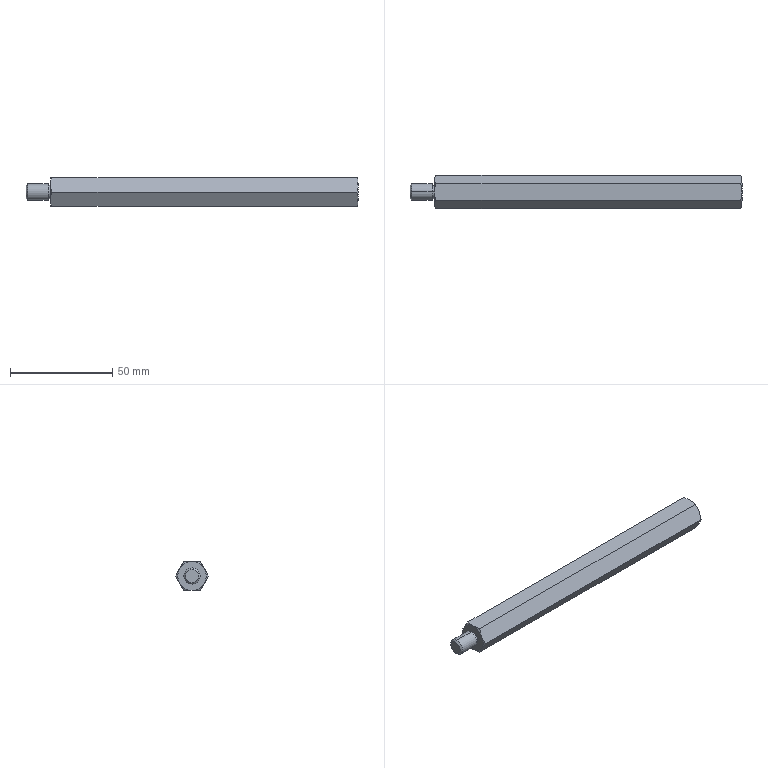Part | STEP file | 0243_007_PLSBWF14-150 | 1 solid | 34 faces | box 162 x 16.166 x 14 mm | volume 25375 mm3 | cone 18 | plane 10 | cylinder 6 | commonest cylinder face diameters 6.4 x2 6.647 x2 8 x2